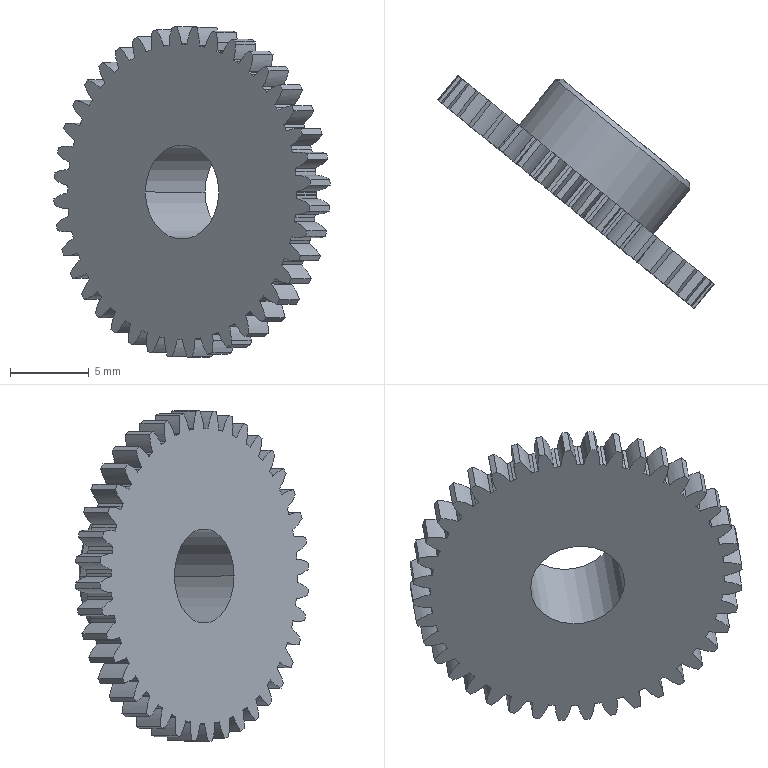Part | SolidWorks | features BaseBody 1 | 1 solid | 297 faces | box 17.541 x 14.79 x 20.982 mm | volume 831.541 mm3 | cylinder 211 | plane 84 | spline 2 | commonest cylinder face diameters 6.076 x85 5.441 x82 21 x40 6 x2 11 x2